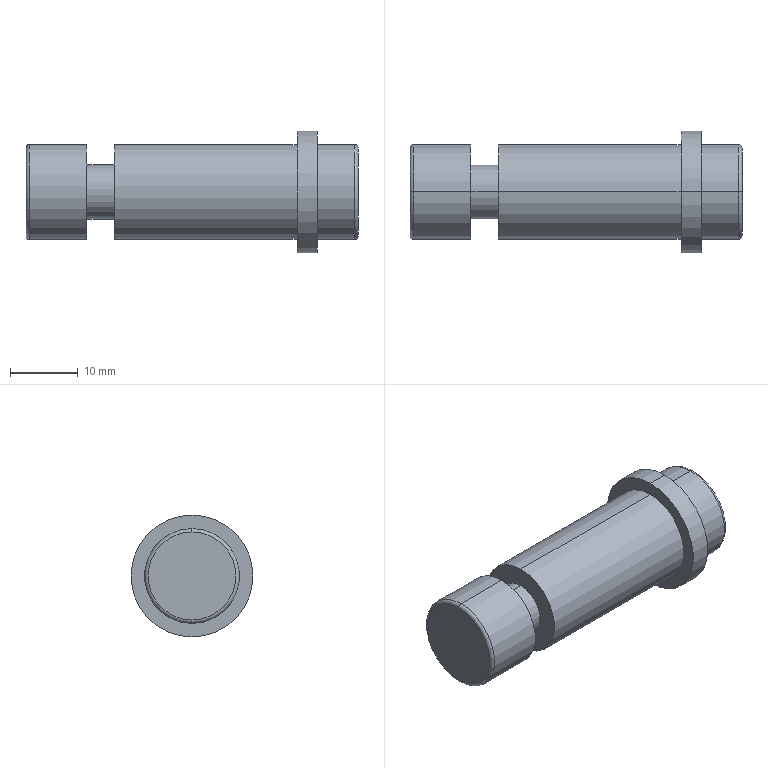Part | SolidWorks | features Fillet 1, Revolution 1 | 1 solid | 20 faces | box 49 x 18 x 18 mm | volume 7425 mm3 | cylinder 10 | plane 6 | torus 4 | commonest cylinder face diameters 14 x6 8 x2 18 x2
STEP:
#1=CARTESIAN_POINT('',(48.5,0.,7.));
#2=VERTEX_POINT('',#1);
#3=CARTESIAN_POINT('',(48.5,0.,-7.));
#4=VERTEX_POINT('',#3);
#5=CARTESIAN_POINT('',(48.5,0.,0.));
#6=DIRECTION('',(-1.,0.,0.));
#7=DIRECTION('',(0.,0.,-1.));
#8=AXIS2_PLACEMENT_3D('',#5,#6,#7);
#9=CIRCLE('',#8,7.);
#10=EDGE_CURVE('',#2,#4,#9,.T.);
#11=ORIENTED_EDGE('',*,*,#10,.F.);
#12=CARTESIAN_POINT('',(49.,0.,6.5));
#13=VERTEX_POINT('',#12);
#14=CARTESIAN_POINT('',(48.5,0.,6.5));
#15=DIRECTION('',(0.,1.,0.));
#16=DIRECTION('',(0.,0.,1.));
#17=AXIS2_PLACEMENT_3D('',#14,#15,#16);
#18=CIRCLE('',#17,0.5);
#19=EDGE_CURVE('',#2,#13,#18,.T.);
#20=ORIENTED_EDGE('',*,*,#19,.T.);
#21=CARTESIAN_POINT('',(49.,0.,-6.5));
#22=VERTEX_POINT('',#21);
#23=CARTESIAN_POINT('',(49.,0.,0.));
#24=DIRECTION('',(1.,0.,0.));
#25=DIRECTION('',(0.,0.,-1.));
#26=AXIS2_PLACEMENT_3D('',#23,#24,#25);
#27=CIRCLE('',#26,6.5);
#28=EDGE_CURVE('',#22,#13,#27,.T.);
#29=ORIENTED_EDGE('',*,*,#28,.F.);
#30=CARTESIAN_POINT('',(48.5,0.,-6.5));
#31=DIRECTION('',(0.,-1.,0.));
#32=DIRECTION('',(0.,0.,-1.));
#33=AXIS2_PLACEMENT_3D('',#30,#31,#32);
#34=CIRCLE('',#33,0.5);
#35=EDGE_CURVE('',#4,#22,#34,.T.);
#36=ORIENTED_EDGE('',*,*,#35,.F.);
#37=EDGE_LOOP('',(#11,#20,#29,#36));
#38=FACE_OUTER_BOUND('',#37,.T.);
#39=CARTESIAN_POINT('',(48.5,0.,0.));
#40=DIRECTION('',(1.,0.,0.));
#41=DIRECTION('',(0.,0.,-1.));
#42=AXIS2_PLACEMENT_3D('',#39,#40,#41);
#43=TOROIDAL_SURFACE('',#42,6.5,0.5);
#44=ADVANCED_FACE('',(#38),#43,.T.);
#45=CARTESIAN_POINT('',(0.5,0.,-7.));
#46=VERTEX_POINT('',#45);
#47=CARTESIAN_POINT('',(0.5,0.,7.));
#48=VERTEX_POINT('',#47);
#49=CARTESIAN_POINT('',(0.5,0.,0.));
#50=DIRECTION('',(1.,0.,0.));
#51=DIRECTION('',(0.,0.,1.));
#52=AXIS2_PLACEMENT_3D('',#49,#50,#51);
#53=CIRCLE('',#52,7.);
#54=EDGE_CURVE('',#46,#48,#53,.T.);
#55=ORIENTED_EDGE('',*,*,#54,.F.);
#56=CARTESIAN_POINT('',(0.,0.,-6.5));
#57=VERTEX_POINT('',#56);
#58=CARTESIAN_POINT('',(0.5,0.,-6.5));
#59=DIRECTION('',(0.,1.,0.));
#60=DIRECTION('',(0.,0.,1.));
#61=AXIS2_PLACEMENT_3D('',#58,#59,#60);
#62=CIRCLE('',#61,0.5);
#63=EDGE_CURVE('',#46,#57,#62,.T.);
#64=ORIENTED_EDGE('',*,*,#63,.T.);
#65=CARTESIAN_POINT('',(0.,0.,6.5));
#66=VERTEX_POINT('',#65);
#67=CARTESIAN_POINT('',(0.,0.,0.));
#68=DIRECTION('',(-1.,0.,0.));
#69=DIRECTION('',(0.,0.,1.));
#70=AXIS2_PLACEMENT_3D('',#67,#68,#69);
#71=CIRCLE('',#70,6.5);
#72=EDGE_CURVE('',#66,#57,#71,.T.);
#73=ORIENTED_EDGE('',*,*,#72,.F.);
#74=CARTESIAN_POINT('',(0.5,0.,6.5));
#75=DIRECTION('',(0.,-1.,0.));
#76=DIRECTION('',(0.,0.,-1.));
#77=AXIS2_PLACEMENT_3D('',#74,#75,#76);
#78=CIRCLE('',#77,0.5);
#79=EDGE_CURVE('',#48,#66,#78,.T.);
#80=ORIENTED_EDGE('',*,*,#79,.F.);
#81=EDGE_LOOP('',(#55,#64,#73,#80));
#82=FACE_OUTER_BOUND('',#81,.T.);
#83=CARTESIAN_POINT('',(0.5,0.,0.));
#84=DIRECTION('',(-1.,0.,0.));
#85=DIRECTION('',(0.,0.,1.));
#86=AXIS2_PLACEMENT_3D('',#83,#84,#85);
#87=TOROIDAL_SURFACE('',#86,6.5,0.5);
#88=ADVANCED_FACE('',(#82),#87,.T.);
#89=CARTESIAN_POINT('',(43.,0.,-7.));
#90=VERTEX_POINT('',#89);
#91=CARTESIAN_POINT('',(43.,0.,7.));
#92=VERTEX_POINT('',#91);
#93=CARTESIAN_POINT('',(43.,0.,0.));
#94=DIRECTION('',(1.,0.,0.));
#95=DIRECTION('',(0.,0.,-1.));
#96=AXIS2_PLACEMENT_3D('',#93,#94,#95);
#97=CIRCLE('',#96,7.);
#98=EDGE_CURVE('',#90,#92,#97,.T.);
#99=ORIENTED_EDGE('',*,*,#98,.T.);
#100=CARTESIAN_POINT('',(49.,0.,7.));
#101=DIRECTION('',(1.,0.,0.));
#102=VECTOR('',#101,1000.);
#103=LINE('',#100,#102);
#104=EDGE_CURVE('',#92,#2,#103,.T.);
#105=ORIENTED_EDGE('',*,*,#104,.T.);
#106=ORIENTED_EDGE('',*,*,#10,.T.);
#107=CARTESIAN_POINT('',(49.,0.,-7.));
#108=DIRECTION('',(1.,0.,0.));
#109=VECTOR('',#108,1000.);
#110=LINE('',#107,#109);
#111=EDGE_CURVE('',#90,#4,#110,.T.);
#112=ORIENTED_EDGE('',*,*,#111,.F.);
#113=EDGE_LOOP('',(#99,#105,#106,#112));
#114=FACE_OUTER_BOUND('',#113,.T.);
#115=CARTESIAN_POINT('',(49.,0.,0.));
#116=DIRECTION('',(1.,0.,0.));
#117=DIRECTION('',(0.,0.,-1.));
#118=AXIS2_PLACEMENT_3D('',#115,#116,#117);
#119=CYLINDRICAL_SURFACE('',#118,7.);
#120=ADVANCED_FACE('',(#114),#119,.T.);
#121=CARTESIAN_POINT('',(40.,0.,-9.));
#122=VERTEX_POINT('',#121);
#123=CARTESIAN_POINT('',(40.,0.,9.));
#124=VERTEX_POINT('',#123);
#125=CARTESIAN_POINT('',(40.,0.,0.));
#126=DIRECTION('',(1.,0.,0.));
#127=DIRECTION('',(0.,0.,-1.));
#128=AXIS2_PLACEMENT_3D('',#125,#126,#127);
#129=CIRCLE('',#128,9.);
#130=EDGE_CURVE('',#122,#124,#129,.T.);
#131=ORIENTED_EDGE('',*,*,#130,.T.);
#132=CARTESIAN_POINT('',(43.,0.,9.));
#133=VERTEX_POINT('',#132);
#134=CARTESIAN_POINT('',(49.,0.,9.));
#135=DIRECTION('',(1.,0.,0.));
#136=VECTOR('',#135,1000.);
#137=LINE('',#134,#136);
#138=EDGE_CURVE('',#124,#133,#137,.T.);
#139=ORIENTED_EDGE('',*,*,#138,.T.);
#140=CARTESIAN_POINT('',(43.,0.,-9.));
#141=VERTEX_POINT('',#140);
#142=CARTESIAN_POINT('',(43.,0.,0.));
#143=DIRECTION('',(1.,0.,0.));
#144=DIRECTION('',(0.,0.,-1.));
#145=AXIS2_PLACEMENT_3D('',#142,#143,#144);
#146=CIRCLE('',#145,9.);
#147=EDGE_CURVE('',#141,#133,#146,.T.);
#148=ORIENTED_EDGE('',*,*,#147,.F.);
#149=CARTESIAN_POINT('',(49.,0.,-9.));
#150=DIRECTION('',(1.,0.,0.));
#151=VECTOR('',#150,1000.);
#152=LINE('',#149,#151);
#153=EDGE_CURVE('',#122,#141,#152,.T.);
#154=ORIENTED_EDGE('',*,*,#153,.F.);
#155=EDGE_LOOP('',(#131,#139,#148,#154));
#156=FACE_OUTER_BOUND('',#155,.T.);
#157=CARTESIAN_POINT('',(49.,0.,0.));
#158=DIRECTION('',(1.,0.,0.));
#159=DIRECTION('',(0.,0.,-1.));
#160=AXIS2_PLACEMENT_3D('',#157,#158,#159);
#161=CYLINDRICAL_SURFACE('',#160,9.);
#162=ADVANCED_FACE('',(#156),#161,.T.);
#163=CARTESIAN_POINT('',(13.,0.,-7.));
#164=VERTEX_POINT('',#163);
#165=CARTESIAN_POINT('',(13.,0.,7.));
#166=VERTEX_POINT('',#165);
#167=CARTESIAN_POINT('',(13.,0.,0.));
#168=DIRECTION('',(1.,0.,0.));
#169=DIRECTION('',(0.,0.,-1.));
#170=AXIS2_PLACEMENT_3D('',#167,#168,#169);
#171=CIRCLE('',#170,7.);
#172=EDGE_CURVE('',#164,#166,#171,.T.);
#173=ORIENTED_EDGE('',*,*,#172,.T.);
#174=CARTESIAN_POINT('',(40.,0.,7.));
#175=VERTEX_POINT('',#174);
#176=CARTESIAN_POINT('',(49.,0.,7.));
#177=DIRECTION('',(1.,0.,0.));
#178=VECTOR('',#177,1000.);
#179=LINE('',#176,#178);
#180=EDGE_CURVE('',#166,#175,#179,.T.);
#181=ORIENTED_EDGE('',*,*,#180,.T.);
#182=CARTESIAN_POINT('',(40.,0.,-7.));
#183=VERTEX_POINT('',#182);
#184=CARTESIAN_POINT('',(40.,0.,0.));
#185=DIRECTION('',(1.,0.,0.));
#186=DIRECTION('',(0.,0.,-1.));
#187=AXIS2_PLACEMENT_3D('',#184,#185,#186);
#188=CIRCLE('',#187,7.);
#189=EDGE_CURVE('',#183,#175,#188,.T.);
#190=ORIENTED_EDGE('',*,*,#189,.F.);
#191=CARTESIAN_POINT('',(49.,0.,-7.));
#192=DIRECTION('',(1.,0.,0.));
#193=VECTOR('',#192,1000.);
#194=LINE('',#191,#193);
#195=EDGE_CURVE('',#164,#183,#194,.T.);
#196=ORIENTED_EDGE('',*,*,#195,.F.);
#197=EDGE_LOOP('',(#173,#181,#190,#196));
#198=FACE_OUTER_BOUND('',#197,.T.);
#199=CARTESIAN_POINT('',(49.,0.,0.));
#200=DIRECTION('',(1.,0.,0.));
#201=DIRECTION('',(0.,0.,-1.));
#202=AXIS2_PLACEMENT_3D('',#199,#200,#201);
#203=CYLINDRICAL_SURFACE('',#202,7.);
#204=ADVANCED_FACE('',(#198),#203,.T.);
#205=CARTESIAN_POINT('',(9.,0.,-4.));
#206=VERTEX_POINT('',#205);
#207=CARTESIAN_POINT('',(9.,0.,4.));
#208=VERTEX_POINT('',#207);
#209=CARTESIAN_POINT('',(9.,0.,0.));
#210=DIRECTION('',(1.,0.,0.));
#211=DIRECTION('',(0.,0.,-1.));
#212=AXIS2_PLACEMENT_3D('',#209,#210,#211);
#213=CIRCLE('',#212,4.);
#214=EDGE_CURVE('',#206,#208,#213,.T.);
#215=ORIENTED_EDGE('',*,*,#214,.T.);
#216=CARTESIAN_POINT('',(13.,0.,4.));
#217=VERTEX_POINT('',#216);
#218=CARTESIAN_POINT('',(49.,0.,4.));
#219=DIRECTION('',(1.,0.,0.));
#220=VECTOR('',#219,1000.);
#221=LINE('',#218,#220);
#222=EDGE_CURVE('',#208,#217,#221,.T.);
#223=ORIENTED_EDGE('',*,*,#222,.T.);
#224=CARTESIAN_POINT('',(13.,0.,-4.));
#225=VERTEX_POINT('',#224);
#226=CARTESIAN_POINT('',(13.,0.,0.));
#227=DIRECTION('',(1.,0.,0.));
#228=DIRECTION('',(0.,0.,-1.));
#229=AXIS2_PLACEMENT_3D('',#226,#227,#228);
#230=CIRCLE('',#229,4.);
#231=EDGE_CURVE('',#225,#217,#230,.T.);
#232=ORIENTED_EDGE('',*,*,#231,.F.);
#233=CARTESIAN_POINT('',(49.,0.,-4.));
#234=DIRECTION('',(1.,0.,0.));
#235=VECTOR('',#234,1000.);
#236=LINE('',#233,#235);
#237=EDGE_CURVE('',#206,#225,#236,.T.);
#238=ORIENTED_EDGE('',*,*,#237,.F.);
#239=EDGE_LOOP('',(#215,#223,#232,#238));
#240=FACE_OUTER_BOUND('',#239,.T.);
#241=CARTESIAN_POINT('',(49.,0.,0.));
#242=DIRECTION('',(1.,0.,0.));
#243=DIRECTION('',(0.,0.,-1.));
#244=AXIS2_PLACEMENT_3D('',#241,#242,#243);
#245=CYLINDRICAL_SURFACE('',#244,4.);
#246=ADVANCED_FACE('',(#240),#245,.T.);
#247=ORIENTED_EDGE('',*,*,#54,.T.);
#248=CARTESIAN_POINT('',(9.,0.,7.));
#249=VERTEX_POINT('',#248);
#250=CARTESIAN_POINT('',(49.,0.,7.));
#251=DIRECTION('',(1.,0.,0.));
#252=VECTOR('',#251,1000.);
#253=LINE('',#250,#252);
#254=EDGE_CURVE('',#48,#249,#253,.T.);
#255=ORIENTED_EDGE('',*,*,#254,.T.);
#256=CARTESIAN_POINT('',(9.,0.,-7.));
#257=VERTEX_POINT('',#256);
#258=CARTESIAN_POINT('',(9.,0.,0.));
#259=DIRECTION('',(1.,0.,0.));
#260=DIRECTION('',(0.,0.,-1.));
#261=AXIS2_PLACEMENT_3D('',#258,#259,#260);
#262=CIRCLE('',#261,7.);
#263=EDGE_CURVE('',#257,#249,#262,.T.);
#264=ORIENTED_EDGE('',*,*,#263,.F.);
#265=CARTESIAN_POINT('',(49.,0.,-7.));
#266=DIRECTION('',(1.,0.,0.));
#267=VECTOR('',#266,1000.);
#268=LINE('',#265,#267);
#269=EDGE_CURVE('',#46,#257,#268,.T.);
#270=ORIENTED_EDGE('',*,*,#269,.F.);
#271=EDGE_LOOP('',(#247,#255,#264,#270));
#272=FACE_OUTER_BOUND('',#271,.T.);
#273=CARTESIAN_POINT('',(49.,0.,0.));
#274=DIRECTION('',(1.,0.,0.));
#275=DIRECTION('',(0.,0.,-1.));
#276=AXIS2_PLACEMENT_3D('',#273,#274,#275);
#277=CYLINDRICAL_SURFACE('',#276,7.);
#278=ADVANCED_FACE('',(#272),#277,.T.);
#279=ORIENTED_EDGE('',*,*,#72,.T.);
#280=CARTESIAN_POINT('',(0.,0.,0.));
#281=DIRECTION('',(-1.,0.,0.));
#282=DIRECTION('',(0.,0.,1.));
#283=AXIS2_PLACEMENT_3D('',#280,#281,#282);
#284=CIRCLE('',#283,6.5);
#285=EDGE_CURVE('',#57,#66,#284,.T.);
#286=ORIENTED_EDGE('',*,*,#285,.T.);
#287=EDGE_LOOP('',(#279,#286));
#288=FACE_OUTER_BOUND('',#287,.T.);
#289=CARTESIAN_POINT('',(0.,0.,0.));
#290=DIRECTION('',(-1.,0.,0.));
#291=DIRECTION('',(0.,0.,1.));
#292=AXIS2_PLACEMENT_3D('',#289,#290,#291);
#293=PLANE('',#292);
#294=ADVANCED_FACE('',(#288),#293,.T.);
#295=ORIENTED_EDGE('',*,*,#254,.F.);
#296=CARTESIAN_POINT('',(0.5,0.,0.));
#297=DIRECTION('',(1.,0.,0.));
#298=DIRECTION('',(0.,0.,1.));
#299=AXIS2_PLACEMENT_3D('',#296,#297,#298);
#300=CIRCLE('',#299,7.);
#301=EDGE_CURVE('',#48,#46,#300,.T.);
#302=ORIENTED_EDGE('',*,*,#301,.T.);
#303=ORIENTED_EDGE('',*,*,#269,.T.);
#304=CARTESIAN_POINT('',(9.,0.,0.));
#305=DIRECTION('',(1.,0.,0.));
#306=DIRECTION('',(0.,0.,-1.));
#307=AXIS2_PLACEMENT_3D('',#304,#305,#306);
#308=CIRCLE('',#307,7.);
#309=EDGE_CURVE('',#249,#257,#308,.T.);
#310=ORIENTED_EDGE('',*,*,#309,.F.);
#311=EDGE_LOOP('',(#295,#302,#303,#310));
#312=FACE_OUTER_BOUND('',#311,.T.);
#313=CARTESIAN_POINT('',(49.,0.,0.));
#314=DIRECTION('',(1.,0.,0.));
#315=DIRECTION('',(0.,0.,-1.));
#316=AXIS2_PLACEMENT_3D('',#313,#314,#315);
#317=CYLINDRICAL_SURFACE('',#316,7.);
#318=ADVANCED_FACE('',(#312),#317,.T.);
#319=ORIENTED_EDGE('',*,*,#263,.T.);
#320=ORIENTED_EDGE('',*,*,#309,.T.);
#321=EDGE_LOOP('',(#319,#320));
#322=FACE_OUTER_BOUND('',#321,.T.);
#323=ORIENTED_EDGE('',*,*,#214,.F.);
#324=CARTESIAN_POINT('',(9.,0.,0.));
#325=DIRECTION('',(1.,0.,0.));
#326=DIRECTION('',(0.,0.,-1.));
#327=AXIS2_PLACEMENT_3D('',#324,#325,#326);
#328=CIRCLE('',#327,4.);
#329=EDGE_CURVE('',#208,#206,#328,.T.);
#330=ORIENTED_EDGE('',*,*,#329,.F.);
#331=EDGE_LOOP('',(#323,#330));
#332=FACE_BOUND('',#331,.T.);
#333=CARTESIAN_POINT('',(9.,7.,0.));
#334=DIRECTION('',(1.,0.,0.));
#335=DIRECTION('',(0.,0.,-1.));
#336=AXIS2_PLACEMENT_3D('',#333,#334,#335);
#337=PLANE('',#336);
#338=ADVANCED_FACE('',(#322,#332),#337,.T.);
#339=ORIENTED_EDGE('',*,*,#222,.F.);
#340=ORIENTED_EDGE('',*,*,#329,.T.);
#341=ORIENTED_EDGE('',*,*,#237,.T.);
#342=CARTESIAN_POINT('',(13.,0.,0.));
#343=DIRECTION('',(1.,0.,0.));
#344=DIRECTION('',(0.,0.,-1.));
#345=AXIS2_PLACEMENT_3D('',#342,#343,#344);
#346=CIRCLE('',#345,4.);
#347=EDGE_CURVE('',#217,#225,#346,.T.);
#348=ORIENTED_EDGE('',*,*,#347,.F.);
#349=EDGE_LOOP('',(#339,#340,#341,#348));
#350=FACE_OUTER_BOUND('',#349,.T.);
#351=CARTESIAN_POINT('',(49.,0.,0.));
#352=DIRECTION('',(1.,0.,0.));
#353=DIRECTION('',(0.,0.,-1.));
#354=AXIS2_PLACEMENT_3D('',#351,#352,#353);
#355=CYLINDRICAL_SURFACE('',#354,4.);
#356=ADVANCED_FACE('',(#350),#355,.T.);
#357=ORIENTED_EDGE('',*,*,#231,.T.);
#358=ORIENTED_EDGE('',*,*,#347,.T.);
#359=EDGE_LOOP('',(#357,#358));
#360=FACE_BOUND('',#359,.T.);
#361=ORIENTED_EDGE('',*,*,#172,.F.);
#362=CARTESIAN_POINT('',(13.,0.,0.));
#363=DIRECTION('',(1.,0.,0.));
#364=DIRECTION('',(0.,0.,-1.));
#365=AXIS2_PLACEMENT_3D('',#362,#363,#364);
#366=CIRCLE('',#365,7.);
#367=EDGE_CURVE('',#166,#164,#366,.T.);
#368=ORIENTED_EDGE('',*,*,#367,.F.);
#369=EDGE_LOOP('',(#361,#368));
#370=FACE_OUTER_BOUND('',#369,.T.);
#371=CARTESIAN_POINT('',(13.,4.,0.));
#372=DIRECTION('',(-1.,0.,0.));
#373=DIRECTION('',(0.,0.,1.));
#374=AXIS2_PLACEMENT_3D('',#371,#372,#373);
#375=PLANE('',#374);
#376=ADVANCED_FACE('',(#360,#370),#375,.T.);
#377=ORIENTED_EDGE('',*,*,#180,.F.);
#378=ORIENTED_EDGE('',*,*,#367,.T.);
#379=ORIENTED_EDGE('',*,*,#195,.T.);
#380=CARTESIAN_POINT('',(40.,0.,0.));
#381=DIRECTION('',(1.,0.,0.));
#382=DIRECTION('',(0.,0.,-1.));
#383=AXIS2_PLACEMENT_3D('',#380,#381,#382);
#384=CIRCLE('',#383,7.);
#385=EDGE_CURVE('',#175,#183,#384,.T.);
#386=ORIENTED_EDGE('',*,*,#385,.F.);
#387=EDGE_LOOP('',(#377,#378,#379,#386));
#388=FACE_OUTER_BOUND('',#387,.T.);
#389=CARTESIAN_POINT('',(49.,0.,0.));
#390=DIRECTION('',(1.,0.,0.));
#391=DIRECTION('',(0.,0.,-1.));
#392=AXIS2_PLACEMENT_3D('',#389,#390,#391);
#393=CYLINDRICAL_SURFACE('',#392,7.);
#394=ADVANCED_FACE('',(#388),#393,.T.);
#395=ORIENTED_EDGE('',*,*,#189,.T.);
#396=ORIENTED_EDGE('',*,*,#385,.T.);
#397=EDGE_LOOP('',(#395,#396));
#398=FACE_BOUND('',#397,.T.);
#399=ORIENTED_EDGE('',*,*,#130,.F.);
#400=CARTESIAN_POINT('',(40.,0.,0.));
#401=DIRECTION('',(1.,0.,0.));
#402=DIRECTION('',(0.,0.,-1.));
#403=AXIS2_PLACEMENT_3D('',#400,#401,#402);
#404=CIRCLE('',#403,9.);
#405=EDGE_CURVE('',#124,#122,#404,.T.);
#406=ORIENTED_EDGE('',*,*,#405,.F.);
#407=EDGE_LOOP('',(#399,#406));
#408=FACE_OUTER_BOUND('',#407,.T.);
#409=CARTESIAN_POINT('',(40.,7.,0.));
#410=DIRECTION('',(-1.,0.,0.));
#411=DIRECTION('',(0.,0.,1.));
#412=AXIS2_PLACEMENT_3D('',#409,#410,#411);
#413=PLANE('',#412);
#414=ADVANCED_FACE('',(#398,#408),#413,.T.);
#415=ORIENTED_EDGE('',*,*,#138,.F.);
#416=ORIENTED_EDGE('',*,*,#405,.T.);
#417=ORIENTED_EDGE('',*,*,#153,.T.);
#418=CARTESIAN_POINT('',(43.,0.,0.));
#419=DIRECTION('',(1.,0.,0.));
#420=DIRECTION('',(0.,0.,-1.));
#421=AXIS2_PLACEMENT_3D('',#418,#419,#420);
#422=CIRCLE('',#421,9.);
#423=EDGE_CURVE('',#133,#141,#422,.T.);
#424=ORIENTED_EDGE('',*,*,#423,.F.);
#425=EDGE_LOOP('',(#415,#416,#417,#424));
#426=FACE_OUTER_BOUND('',#425,.T.);
#427=CARTESIAN_POINT('',(49.,0.,0.));
#428=DIRECTION('',(1.,0.,0.));
#429=DIRECTION('',(0.,0.,-1.));
#430=AXIS2_PLACEMENT_3D('',#427,#428,#429);
#431=CYLINDRICAL_SURFACE('',#430,9.);
#432=ADVANCED_FACE('',(#426),#431,.T.);
#433=ORIENTED_EDGE('',*,*,#147,.T.);
#434=ORIENTED_EDGE('',*,*,#423,.T.);
#435=EDGE_LOOP('',(#433,#434));
#436=FACE_OUTER_BOUND('',#435,.T.);
#437=ORIENTED_EDGE('',*,*,#98,.F.);
#438=CARTESIAN_POINT('',(43.,0.,0.));
#439=DIRECTION('',(1.,0.,0.));
#440=DIRECTION('',(0.,0.,-1.));
#441=AXIS2_PLACEMENT_3D('',#438,#439,#440);
#442=CIRCLE('',#441,7.);
#443=EDGE_CURVE('',#92,#90,#442,.T.);
#444=ORIENTED_EDGE('',*,*,#443,.F.);
#445=EDGE_LOOP('',(#437,#444));
#446=FACE_BOUND('',#445,.T.);
#447=CARTESIAN_POINT('',(43.,9.,0.));
#448=DIRECTION('',(1.,0.,0.));
#449=DIRECTION('',(0.,0.,-1.));
#450=AXIS2_PLACEMENT_3D('',#447,#448,#449);
#451=PLANE('',#450);
#452=ADVANCED_FACE('',(#436,#446),#451,.T.);
#453=ORIENTED_EDGE('',*,*,#104,.F.);
#454=ORIENTED_EDGE('',*,*,#443,.T.);
#455=ORIENTED_EDGE('',*,*,#111,.T.);
#456=CARTESIAN_POINT('',(48.5,0.,0.));
#457=DIRECTION('',(-1.,0.,0.));
#458=DIRECTION('',(0.,0.,-1.));
#459=AXIS2_PLACEMENT_3D('',#456,#457,#458);
#460=CIRCLE('',#459,7.);
#461=EDGE_CURVE('',#4,#2,#460,.T.);
#462=ORIENTED_EDGE('',*,*,#461,.T.);
#463=EDGE_LOOP('',(#453,#454,#455,#462));
#464=FACE_OUTER_BOUND('',#463,.T.);
#465=CARTESIAN_POINT('',(49.,0.,0.));
#466=DIRECTION('',(1.,0.,0.));
#467=DIRECTION('',(0.,0.,-1.));
#468=AXIS2_PLACEMENT_3D('',#465,#466,#467);
#469=CYLINDRICAL_SURFACE('',#468,7.);
#470=ADVANCED_FACE('',(#464),#469,.T.);
#471=ORIENTED_EDGE('',*,*,#28,.T.);
#472=CARTESIAN_POINT('',(49.,0.,0.));
#473=DIRECTION('',(1.,0.,0.));
#474=DIRECTION('',(0.,0.,-1.));
#475=AXIS2_PLACEMENT_3D('',#472,#473,#474);
#476=CIRCLE('',#475,6.5);
#477=EDGE_CURVE('',#13,#22,#476,.T.);
#478=ORIENTED_EDGE('',*,*,#477,.T.);
#479=EDGE_LOOP('',(#471,#478));
#480=FACE_OUTER_BOUND('',#479,.T.);
#481=CARTESIAN_POINT('',(49.,7.,0.));
#482=DIRECTION('',(1.,0.,0.));
#483=DIRECTION('',(0.,0.,-1.));
#484=AXIS2_PLACEMENT_3D('',#481,#482,#483);
#485=PLANE('',#484);
#486=ADVANCED_FACE('',(#480),#485,.T.);
#487=ORIENTED_EDGE('',*,*,#63,.F.);
#488=ORIENTED_EDGE('',*,*,#301,.F.);
#489=ORIENTED_EDGE('',*,*,#79,.T.);
#490=ORIENTED_EDGE('',*,*,#285,.F.);
#491=EDGE_LOOP('',(#487,#488,#489,#490));
#492=FACE_OUTER_BOUND('',#491,.T.);
#493=CARTESIAN_POINT('',(0.5,0.,0.));
#494=DIRECTION('',(-1.,0.,0.));
#495=DIRECTION('',(0.,0.,1.));
#496=AXIS2_PLACEMENT_3D('',#493,#494,#495);
#497=TOROIDAL_SURFACE('',#496,6.5,0.5);
#498=ADVANCED_FACE('',(#492),#497,.T.);
#499=ORIENTED_EDGE('',*,*,#19,.F.);
#500=ORIENTED_EDGE('',*,*,#461,.F.);
#501=ORIENTED_EDGE('',*,*,#35,.T.);
#502=ORIENTED_EDGE('',*,*,#477,.F.);
#503=EDGE_LOOP('',(#499,#500,#501,#502));
#504=FACE_OUTER_BOUND('',#503,.T.);
#505=CARTESIAN_POINT('',(48.5,0.,0.));
#506=DIRECTION('',(1.,0.,0.));
#507=DIRECTION('',(0.,0.,-1.));
#508=AXIS2_PLACEMENT_3D('',#505,#506,#507);
#509=TOROIDAL_SURFACE('',#508,6.5,0.5);
#510=ADVANCED_FACE('',(#504),#509,.T.);
#511=CLOSED_SHELL('',(#44,#88,#120,#162,#204,#246,#278,#294,#318,#338,#356,#376,#394,#414,#432,#452,#470,#486,#498,#510));
#512=MANIFOLD_SOLID_BREP('',#511);
#513=CARTESIAN_POINT('',(0.,0.,0.));
#514=DIRECTION('',(0.,0.,1.));
#515=DIRECTION('',(1.,0.,0.));
#516=AXIS2_PLACEMENT_3D('',#513,#514,#515);
#517=(LENGTH_UNIT()NAMED_UNIT(*)SI_UNIT(.MILLI.,.METRE.));
#518=UNCERTAINTY_MEASURE_WITH_UNIT(LENGTH_MEASURE(0.00001),#517,'','');
#519=(NAMED_UNIT(*)PLANE_ANGLE_UNIT()SI_UNIT($,.RADIAN.));
#520=(NAMED_UNIT(*)SI_UNIT($,.STERADIAN.)SOLID_ANGLE_UNIT());
#521=(GEOMETRIC_REPRESENTATION_CONTEXT(3)GLOBAL_UNCERTAINTY_ASSIGNED_CONTEXT((#518))GLOBAL_UNIT_ASSIGNED_CONTEXT((#517,#519,#520))REPRESENTATION_CONTEXT('',''));
#522=ADVANCED_BREP_SHAPE_REPRESENTATION('',(#512,#516),#521);